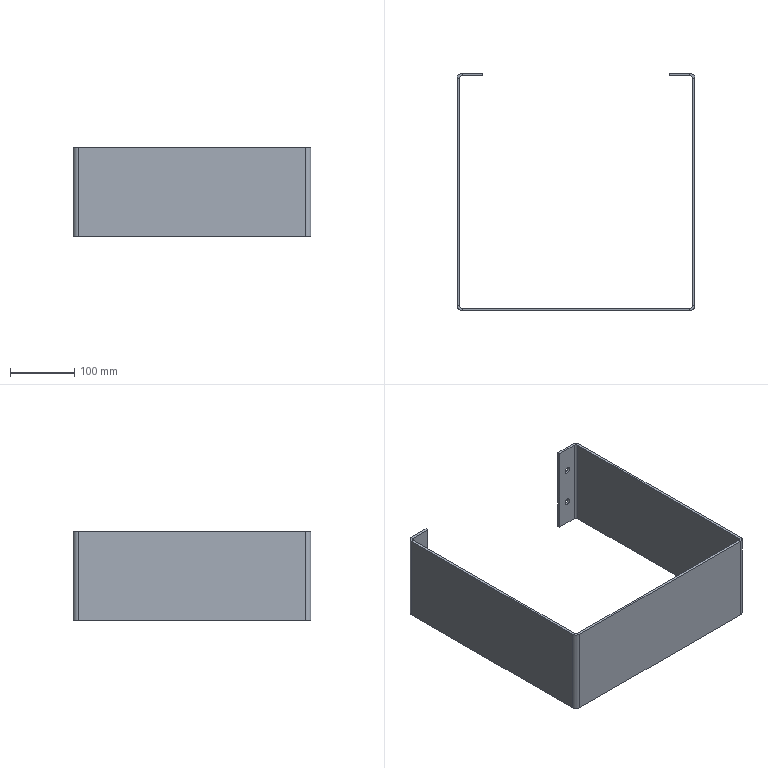Part | SolidWorks | features EdgeFlange 3, FlatPattern 1, ICE 1, SMBaseFlange 1, SheetMetal 1 | 1 solid | 46 faces | box 370 x 370 x 140 mm | volume 650415 mm3 | plane 30 | cylinder 16 | commonest cylinder face diameters 10 x8 8 x4 16 x4
STEP:
#1=CARTESIAN_POINT('',(-162.,366.,25.));
#2=VERTEX_POINT('',#1);
#3=CARTESIAN_POINT('',(-162.,366.,35.));
#4=VERTEX_POINT('',#3);
#5=CARTESIAN_POINT('',(-162.,366.,30.));
#6=DIRECTION('',(0.,1.,0.));
#7=DIRECTION('',(-1.,0.,0.));
#8=AXIS2_PLACEMENT_3D('',#5,#6,#7);
#9=CIRCLE('',#8,5.);
#10=EDGE_CURVE('',#2,#4,#9,.T.);
#11=ORIENTED_EDGE('',*,*,#10,.F.);
#12=CARTESIAN_POINT('',(-162.,370.,25.));
#13=VERTEX_POINT('',#12);
#14=CARTESIAN_POINT('',(-162.,280.,25.));
#15=DIRECTION('',(0.,1.,0.));
#16=VECTOR('',#15,1000.);
#17=LINE('',#14,#16);
#18=EDGE_CURVE('',#2,#13,#17,.T.);
#19=ORIENTED_EDGE('',*,*,#18,.T.);
#20=CARTESIAN_POINT('',(-162.,370.,35.));
#21=VERTEX_POINT('',#20);
#22=CARTESIAN_POINT('',(-162.,370.,30.));
#23=DIRECTION('',(0.,1.,0.));
#24=DIRECTION('',(0.,0.,-1.));
#25=AXIS2_PLACEMENT_3D('',#22,#23,#24);
#26=CIRCLE('',#25,5.);
#27=EDGE_CURVE('',#13,#21,#26,.T.);
#28=ORIENTED_EDGE('',*,*,#27,.T.);
#29=CARTESIAN_POINT('',(-162.,280.,35.));
#30=DIRECTION('',(0.,1.,0.));
#31=VECTOR('',#30,1000.);
#32=LINE('',#29,#31);
#33=EDGE_CURVE('',#4,#21,#32,.T.);
#34=ORIENTED_EDGE('',*,*,#33,.F.);
#35=EDGE_LOOP('',(#11,#19,#28,#34));
#36=FACE_OUTER_BOUND('',#35,.T.);
#37=CARTESIAN_POINT('',(-162.,280.,30.));
#38=DIRECTION('',(0.,1.,0.));
#39=DIRECTION('',(0.,0.,1.));
#40=AXIS2_PLACEMENT_3D('',#37,#38,#39);
#41=CYLINDRICAL_SURFACE('',#40,5.);
#42=ADVANCED_FACE('',(#36),#41,.F.);
#43=CARTESIAN_POINT('',(-162.,366.,-35.));
#44=VERTEX_POINT('',#43);
#45=CARTESIAN_POINT('',(-162.,366.,-25.));
#46=VERTEX_POINT('',#45);
#47=CARTESIAN_POINT('',(-162.,366.,-30.));
#48=DIRECTION('',(0.,1.,0.));
#49=DIRECTION('',(-1.,0.,0.));
#50=AXIS2_PLACEMENT_3D('',#47,#48,#49);
#51=CIRCLE('',#50,5.);
#52=EDGE_CURVE('',#44,#46,#51,.T.);
#53=ORIENTED_EDGE('',*,*,#52,.F.);
#54=CARTESIAN_POINT('',(-162.,370.,-35.));
#55=VERTEX_POINT('',#54);
#56=CARTESIAN_POINT('',(-162.,280.,-35.));
#57=DIRECTION('',(0.,1.,0.));
#58=VECTOR('',#57,1000.);
#59=LINE('',#56,#58);
#60=EDGE_CURVE('',#44,#55,#59,.T.);
#61=ORIENTED_EDGE('',*,*,#60,.T.);
#62=CARTESIAN_POINT('',(-162.,370.,-25.));
#63=VERTEX_POINT('',#62);
#64=CARTESIAN_POINT('',(-162.,370.,-30.));
#65=DIRECTION('',(0.,1.,0.));
#66=DIRECTION('',(0.,0.,1.));
#67=AXIS2_PLACEMENT_3D('',#64,#65,#66);
#68=CIRCLE('',#67,5.);
#69=EDGE_CURVE('',#55,#63,#68,.T.);
#70=ORIENTED_EDGE('',*,*,#69,.T.);
#71=CARTESIAN_POINT('',(-162.,280.,-25.));
#72=DIRECTION('',(0.,1.,0.));
#73=VECTOR('',#72,1000.);
#74=LINE('',#71,#73);
#75=EDGE_CURVE('',#46,#63,#74,.T.);
#76=ORIENTED_EDGE('',*,*,#75,.F.);
#77=EDGE_LOOP('',(#53,#61,#70,#76));
#78=FACE_OUTER_BOUND('',#77,.T.);
#79=CARTESIAN_POINT('',(-162.,280.,-30.));
#80=DIRECTION('',(0.,1.,0.));
#81=DIRECTION('',(0.,0.,1.));
#82=AXIS2_PLACEMENT_3D('',#79,#80,#81);
#83=CYLINDRICAL_SURFACE('',#82,5.);
#84=ADVANCED_FACE('',(#78),#83,.F.);
#85=CARTESIAN_POINT('',(162.,366.,-35.));
#86=VERTEX_POINT('',#85);
#87=CARTESIAN_POINT('',(162.,366.,-25.));
#88=VERTEX_POINT('',#87);
#89=CARTESIAN_POINT('',(162.,366.,-30.));
#90=DIRECTION('',(0.,1.,0.));
#91=DIRECTION('',(-1.,0.,0.));
#92=AXIS2_PLACEMENT_3D('',#89,#90,#91);
#93=CIRCLE('',#92,5.);
#94=EDGE_CURVE('',#86,#88,#93,.T.);
#95=ORIENTED_EDGE('',*,*,#94,.F.);
#96=CARTESIAN_POINT('',(162.,370.,-35.));
#97=VERTEX_POINT('',#96);
#98=CARTESIAN_POINT('',(162.,280.,-35.));
#99=DIRECTION('',(0.,1.,0.));
#100=VECTOR('',#99,1000.);
#101=LINE('',#98,#100);
#102=EDGE_CURVE('',#86,#97,#101,.T.);
#103=ORIENTED_EDGE('',*,*,#102,.T.);
#104=CARTESIAN_POINT('',(162.,370.,-25.));
#105=VERTEX_POINT('',#104);
#106=CARTESIAN_POINT('',(162.,370.,-30.));
#107=DIRECTION('',(0.,1.,0.));
#108=DIRECTION('',(0.,0.,-1.));
#109=AXIS2_PLACEMENT_3D('',#106,#107,#108);
#110=CIRCLE('',#109,5.);
#111=EDGE_CURVE('',#97,#105,#110,.T.);
#112=ORIENTED_EDGE('',*,*,#111,.T.);
#113=CARTESIAN_POINT('',(162.,280.,-25.));
#114=DIRECTION('',(0.,1.,0.));
#115=VECTOR('',#114,1000.);
#116=LINE('',#113,#115);
#117=EDGE_CURVE('',#88,#105,#116,.T.);
#118=ORIENTED_EDGE('',*,*,#117,.F.);
#119=EDGE_LOOP('',(#95,#103,#112,#118));
#120=FACE_OUTER_BOUND('',#119,.T.);
#121=CARTESIAN_POINT('',(162.,280.,-30.));
#122=DIRECTION('',(0.,1.,0.));
#123=DIRECTION('',(0.,0.,1.));
#124=AXIS2_PLACEMENT_3D('',#121,#122,#123);
#125=CYLINDRICAL_SURFACE('',#124,5.);
#126=ADVANCED_FACE('',(#120),#125,.F.);
#127=CARTESIAN_POINT('',(162.,366.,25.));
#128=VERTEX_POINT('',#127);
#129=CARTESIAN_POINT('',(162.,366.,35.));
#130=VERTEX_POINT('',#129);
#131=CARTESIAN_POINT('',(162.,366.,30.));
#132=DIRECTION('',(0.,1.,0.));
#133=DIRECTION('',(-1.,0.,0.));
#134=AXIS2_PLACEMENT_3D('',#131,#132,#133);
#135=CIRCLE('',#134,5.);
#136=EDGE_CURVE('',#128,#130,#135,.T.);
#137=ORIENTED_EDGE('',*,*,#136,.F.);
#138=CARTESIAN_POINT('',(162.,370.,25.));
#139=VERTEX_POINT('',#138);
#140=CARTESIAN_POINT('',(162.,280.,25.));
#141=DIRECTION('',(0.,1.,0.));
#142=VECTOR('',#141,1000.);
#143=LINE('',#140,#142);
#144=EDGE_CURVE('',#128,#139,#143,.T.);
#145=ORIENTED_EDGE('',*,*,#144,.T.);
#146=CARTESIAN_POINT('',(162.,370.,35.));
#147=VERTEX_POINT('',#146);
#148=CARTESIAN_POINT('',(162.,370.,30.));
#149=DIRECTION('',(0.,1.,0.));
#150=DIRECTION('',(0.,0.,1.));
#151=AXIS2_PLACEMENT_3D('',#148,#149,#150);
#152=CIRCLE('',#151,5.);
#153=EDGE_CURVE('',#139,#147,#152,.T.);
#154=ORIENTED_EDGE('',*,*,#153,.T.);
#155=CARTESIAN_POINT('',(162.,280.,35.));
#156=DIRECTION('',(0.,1.,0.));
#157=VECTOR('',#156,1000.);
#158=LINE('',#155,#157);
#159=EDGE_CURVE('',#130,#147,#158,.T.);
#160=ORIENTED_EDGE('',*,*,#159,.F.);
#161=EDGE_LOOP('',(#137,#145,#154,#160));
#162=FACE_OUTER_BOUND('',#161,.T.);
#163=CARTESIAN_POINT('',(162.,280.,30.));
#164=DIRECTION('',(0.,1.,0.));
#165=DIRECTION('',(0.,0.,1.));
#166=AXIS2_PLACEMENT_3D('',#163,#164,#165);
#167=CYLINDRICAL_SURFACE('',#166,5.);
#168=ADVANCED_FACE('',(#162),#167,.F.);
#169=CARTESIAN_POINT('',(181.,362.,70.));
#170=VERTEX_POINT('',#169);
#171=CARTESIAN_POINT('',(185.,362.,70.));
#172=VERTEX_POINT('',#171);
#173=CARTESIAN_POINT('',(181.,362.,70.));
#174=DIRECTION('',(1.,0.,0.));
#175=VECTOR('',#174,1000.);
#176=LINE('',#173,#175);
#177=EDGE_CURVE('',#170,#172,#176,.T.);
#178=ORIENTED_EDGE('',*,*,#177,.F.);
#179=CARTESIAN_POINT('',(181.,8.,70.));
#180=VERTEX_POINT('',#179);
#181=CARTESIAN_POINT('',(181.,4.,70.));
#182=DIRECTION('',(0.,-1.,0.));
#183=VECTOR('',#182,1000.);
#184=LINE('',#181,#183);
#185=EDGE_CURVE('',#170,#180,#184,.T.);
#186=ORIENTED_EDGE('',*,*,#185,.T.);
#187=CARTESIAN_POINT('',(185.,8.,70.));
#188=VERTEX_POINT('',#187);
#189=CARTESIAN_POINT('',(185.,8.,70.));
#190=DIRECTION('',(1.,0.,0.));
#191=VECTOR('',#190,1000.);
#192=LINE('',#189,#191);
#193=EDGE_CURVE('',#180,#188,#192,.T.);
#194=ORIENTED_EDGE('',*,*,#193,.T.);
#195=CARTESIAN_POINT('',(185.,0.,70.));
#196=DIRECTION('',(0.,-1.,0.));
#197=VECTOR('',#196,1000.);
#198=LINE('',#195,#197);
#199=EDGE_CURVE('',#172,#188,#198,.T.);
#200=ORIENTED_EDGE('',*,*,#199,.F.);
#201=EDGE_LOOP('',(#178,#186,#194,#200));
#202=FACE_OUTER_BOUND('',#201,.T.);
#203=CARTESIAN_POINT('',(185.,4.,70.));
#204=DIRECTION('',(0.,0.,-1.));
#205=DIRECTION('',(-1.,0.,0.));
#206=AXIS2_PLACEMENT_3D('',#203,#204,#205);
#207=PLANE('',#206);
#208=ADVANCED_FACE('',(#202),#207,.F.);
#209=CARTESIAN_POINT('',(181.,362.,-70.));
#210=VERTEX_POINT('',#209);
#211=CARTESIAN_POINT('',(185.,362.,-70.));
#212=VERTEX_POINT('',#211);
#213=CARTESIAN_POINT('',(181.,362.,-70.));
#214=DIRECTION('',(1.,0.,0.));
#215=VECTOR('',#214,1000.);
#216=LINE('',#213,#215);
#217=EDGE_CURVE('',#210,#212,#216,.T.);
#218=ORIENTED_EDGE('',*,*,#217,.T.);
#219=CARTESIAN_POINT('',(185.,8.,-70.));
#220=VERTEX_POINT('',#219);
#221=CARTESIAN_POINT('',(185.,0.,-70.));
#222=DIRECTION('',(0.,1.,0.));
#223=VECTOR('',#222,1000.);
#224=LINE('',#221,#223);
#225=EDGE_CURVE('',#220,#212,#224,.T.);
#226=ORIENTED_EDGE('',*,*,#225,.F.);
#227=CARTESIAN_POINT('',(181.,8.,-70.));
#228=VERTEX_POINT('',#227);
#229=CARTESIAN_POINT('',(181.,8.,-70.));
#230=DIRECTION('',(1.,0.,0.));
#231=VECTOR('',#230,1000.);
#232=LINE('',#229,#231);
#233=EDGE_CURVE('',#228,#220,#232,.T.);
#234=ORIENTED_EDGE('',*,*,#233,.F.);
#235=CARTESIAN_POINT('',(181.,370.,-70.));
#236=DIRECTION('',(0.,1.,0.));
#237=VECTOR('',#236,1000.);
#238=LINE('',#235,#237);
#239=EDGE_CURVE('',#228,#210,#238,.T.);
#240=ORIENTED_EDGE('',*,*,#239,.T.);
#241=EDGE_LOOP('',(#218,#226,#234,#240));
#242=FACE_OUTER_BOUND('',#241,.T.);
#243=CARTESIAN_POINT('',(185.,370.,-70.));
#244=DIRECTION('',(0.,0.,1.));
#245=DIRECTION('',(0.,-1.,0.));
#246=AXIS2_PLACEMENT_3D('',#243,#244,#245);
#247=PLANE('',#246);
#248=ADVANCED_FACE('',(#242),#247,.F.);
#249=CARTESIAN_POINT('',(185.,362.,-70.));
#250=DIRECTION('',(0.,0.,1.));
#251=VECTOR('',#250,1000.);
#252=LINE('',#249,#251);
#253=EDGE_CURVE('',#212,#172,#252,.T.);
#254=ORIENTED_EDGE('',*,*,#253,.T.);
#255=ORIENTED_EDGE('',*,*,#199,.T.);
#256=CARTESIAN_POINT('',(185.,8.,70.));
#257=DIRECTION('',(0.,0.,1.));
#258=VECTOR('',#257,1000.);
#259=LINE('',#256,#258);
#260=EDGE_CURVE('',#220,#188,#259,.T.);
#261=ORIENTED_EDGE('',*,*,#260,.F.);
#262=ORIENTED_EDGE('',*,*,#225,.T.);
#263=EDGE_LOOP('',(#254,#255,#261,#262));
#264=FACE_OUTER_BOUND('',#263,.T.);
#265=CARTESIAN_POINT('',(185.,0.,0.));
#266=DIRECTION('',(-1.,0.,0.));
#267=DIRECTION('',(0.,-1.,0.));
#268=AXIS2_PLACEMENT_3D('',#265,#266,#267);
#269=PLANE('',#268);
#270=ADVANCED_FACE('',(#264),#269,.F.);
#271=ORIENTED_EDGE('',*,*,#185,.F.);
#272=CARTESIAN_POINT('',(181.,362.,-70.));
#273=DIRECTION('',(0.,0.,1.));
#274=VECTOR('',#273,1000.);
#275=LINE('',#272,#274);
#276=EDGE_CURVE('',#210,#170,#275,.T.);
#277=ORIENTED_EDGE('',*,*,#276,.F.);
#278=ORIENTED_EDGE('',*,*,#239,.F.);
#279=CARTESIAN_POINT('',(181.,8.,70.));
#280=DIRECTION('',(0.,0.,-1.));
#281=VECTOR('',#280,1000.);
#282=LINE('',#279,#281);
#283=EDGE_CURVE('',#180,#228,#282,.T.);
#284=ORIENTED_EDGE('',*,*,#283,.F.);
#285=EDGE_LOOP('',(#271,#277,#278,#284));
#286=FACE_OUTER_BOUND('',#285,.T.);
#287=CARTESIAN_POINT('',(181.,0.,0.));
#288=DIRECTION('',(-1.,0.,0.));
#289=DIRECTION('',(0.,-1.,0.));
#290=AXIS2_PLACEMENT_3D('',#287,#288,#289);
#291=PLANE('',#290);
#292=ADVANCED_FACE('',(#286),#291,.T.);
#293=CARTESIAN_POINT('',(-181.,362.,70.));
#294=VERTEX_POINT('',#293);
#295=CARTESIAN_POINT('',(-185.,362.,70.));
#296=VERTEX_POINT('',#295);
#297=CARTESIAN_POINT('',(-181.,362.,70.));
#298=DIRECTION('',(-1.,0.,0.));
#299=VECTOR('',#298,1000.);
#300=LINE('',#297,#299);
#301=EDGE_CURVE('',#294,#296,#300,.T.);
#302=ORIENTED_EDGE('',*,*,#301,.T.);
#303=CARTESIAN_POINT('',(-185.,8.,70.));
#304=VERTEX_POINT('',#303);
#305=CARTESIAN_POINT('',(-185.,0.,70.));
#306=DIRECTION('',(0.,1.,0.));
#307=VECTOR('',#306,1000.);
#308=LINE('',#305,#307);
#309=EDGE_CURVE('',#304,#296,#308,.T.);
#310=ORIENTED_EDGE('',*,*,#309,.F.);
#311=CARTESIAN_POINT('',(-181.,8.,70.));
#312=VERTEX_POINT('',#311);
#313=CARTESIAN_POINT('',(-181.,8.,70.));
#314=DIRECTION('',(-1.,0.,0.));
#315=VECTOR('',#314,1000.);
#316=LINE('',#313,#315);
#317=EDGE_CURVE('',#312,#304,#316,.T.);
#318=ORIENTED_EDGE('',*,*,#317,.F.);
#319=CARTESIAN_POINT('',(-181.,4.,70.));
#320=DIRECTION('',(0.,1.,0.));
#321=VECTOR('',#320,1000.);
#322=LINE('',#319,#321);
#323=EDGE_CURVE('',#312,#294,#322,.T.);
#324=ORIENTED_EDGE('',*,*,#323,.T.);
#325=EDGE_LOOP('',(#302,#310,#318,#324));
#326=FACE_OUTER_BOUND('',#325,.T.);
#327=CARTESIAN_POINT('',(-185.,4.,70.));
#328=DIRECTION('',(0.,0.,-1.));
#329=DIRECTION('',(-1.,0.,0.));
#330=AXIS2_PLACEMENT_3D('',#327,#328,#329);
#331=PLANE('',#330);
#332=ADVANCED_FACE('',(#326),#331,.F.);
#333=CARTESIAN_POINT('',(-181.,362.,-70.));
#334=VERTEX_POINT('',#333);
#335=CARTESIAN_POINT('',(-185.,362.,-70.));
#336=VERTEX_POINT('',#335);
#337=CARTESIAN_POINT('',(-181.,362.,-70.));
#338=DIRECTION('',(-1.,0.,0.));
#339=VECTOR('',#338,1000.);
#340=LINE('',#337,#339);
#341=EDGE_CURVE('',#334,#336,#340,.T.);
#342=ORIENTED_EDGE('',*,*,#341,.F.);
#343=CARTESIAN_POINT('',(-181.,8.,-70.));
#344=VERTEX_POINT('',#343);
#345=CARTESIAN_POINT('',(-181.,370.,-70.));
#346=DIRECTION('',(0.,-1.,0.));
#347=VECTOR('',#346,1000.);
#348=LINE('',#345,#347);
#349=EDGE_CURVE('',#334,#344,#348,.T.);
#350=ORIENTED_EDGE('',*,*,#349,.T.);
#351=CARTESIAN_POINT('',(-185.,8.,-70.));
#352=VERTEX_POINT('',#351);
#353=CARTESIAN_POINT('',(-185.,8.,-70.));
#354=DIRECTION('',(-1.,0.,0.));
#355=VECTOR('',#354,1000.);
#356=LINE('',#353,#355);
#357=EDGE_CURVE('',#344,#352,#356,.T.);
#358=ORIENTED_EDGE('',*,*,#357,.T.);
#359=CARTESIAN_POINT('',(-185.,0.,-70.));
#360=DIRECTION('',(0.,-1.,0.));
#361=VECTOR('',#360,1000.);
#362=LINE('',#359,#361);
#363=EDGE_CURVE('',#336,#352,#362,.T.);
#364=ORIENTED_EDGE('',*,*,#363,.F.);
#365=EDGE_LOOP('',(#342,#350,#358,#364));
#366=FACE_OUTER_BOUND('',#365,.T.);
#367=CARTESIAN_POINT('',(-185.,370.,-70.));
#368=DIRECTION('',(0.,0.,1.));
#369=DIRECTION('',(0.,-1.,0.));
#370=AXIS2_PLACEMENT_3D('',#367,#368,#369);
#371=PLANE('',#370);
#372=ADVANCED_FACE('',(#366),#371,.F.);
#373=ORIENTED_EDGE('',*,*,#309,.T.);
#374=CARTESIAN_POINT('',(-185.,362.,70.));
#375=DIRECTION('',(0.,0.,-1.));
#376=VECTOR('',#375,1000.);
#377=LINE('',#374,#376);
#378=EDGE_CURVE('',#296,#336,#377,.T.);
#379=ORIENTED_EDGE('',*,*,#378,.T.);
#380=ORIENTED_EDGE('',*,*,#363,.T.);
#381=CARTESIAN_POINT('',(-185.,8.,0.));
#382=DIRECTION('',(0.,0.,1.));
#383=VECTOR('',#382,1000.);
#384=LINE('',#381,#383);
#385=EDGE_CURVE('',#352,#304,#384,.T.);
#386=ORIENTED_EDGE('',*,*,#385,.T.);
#387=EDGE_LOOP('',(#373,#379,#380,#386));
#388=FACE_OUTER_BOUND('',#387,.T.);
#389=CARTESIAN_POINT('',(-185.,0.,0.));
#390=DIRECTION('',(-1.,0.,0.));
#391=DIRECTION('',(0.,-1.,0.));
#392=AXIS2_PLACEMENT_3D('',#389,#390,#391);
#393=PLANE('',#392);
#394=ADVANCED_FACE('',(#388),#393,.T.);
#395=CARTESIAN_POINT('',(-181.,362.,70.));
#396=DIRECTION('',(0.,0.,-1.));
#397=VECTOR('',#396,1000.);
#398=LINE('',#395,#397);
#399=EDGE_CURVE('',#294,#334,#398,.T.);
#400=ORIENTED_EDGE('',*,*,#399,.F.);
#401=ORIENTED_EDGE('',*,*,#323,.F.);
#402=CARTESIAN_POINT('',(-181.,8.,-70.));
#403=DIRECTION('',(0.,0.,1.));
#404=VECTOR('',#403,1000.);
#405=LINE('',#402,#404);
#406=EDGE_CURVE('',#344,#312,#405,.T.);
#407=ORIENTED_EDGE('',*,*,#406,.F.);
#408=ORIENTED_EDGE('',*,*,#349,.F.);
#409=EDGE_LOOP('',(#400,#401,#407,#408));
#410=FACE_OUTER_BOUND('',#409,.T.);
#411=CARTESIAN_POINT('',(-181.,0.,0.));
#412=DIRECTION('',(-1.,0.,0.));
#413=DIRECTION('',(0.,-1.,0.));
#414=AXIS2_PLACEMENT_3D('',#411,#412,#413);
#415=PLANE('',#414);
#416=ADVANCED_FACE('',(#410),#415,.F.);
#417=CARTESIAN_POINT('',(177.,4.,-70.));
#418=VERTEX_POINT('',#417);
#419=CARTESIAN_POINT('',(177.,0.,-70.));
#420=VERTEX_POINT('',#419);
#421=CARTESIAN_POINT('',(177.,4.,-70.));
#422=DIRECTION('',(0.,-1.,0.));
#423=VECTOR('',#422,1000.);
#424=LINE('',#421,#423);
#425=EDGE_CURVE('',#418,#420,#424,.T.);
#426=ORIENTED_EDGE('',*,*,#425,.T.);
#427=CARTESIAN_POINT('',(-177.,0.,-70.));
#428=VERTEX_POINT('',#427);
#429=CARTESIAN_POINT('',(-185.,0.,-70.));
#430=DIRECTION('',(-1.,0.,0.));
#431=VECTOR('',#430,1000.);
#432=LINE('',#429,#431);
#433=EDGE_CURVE('',#420,#428,#432,.T.);
#434=ORIENTED_EDGE('',*,*,#433,.T.);
#435=CARTESIAN_POINT('',(-177.,4.,-70.));
#436=VERTEX_POINT('',#435);
#437=CARTESIAN_POINT('',(-177.,4.,-70.));
#438=DIRECTION('',(0.,-1.,0.));
#439=VECTOR('',#438,1000.);
#440=LINE('',#437,#439);
#441=EDGE_CURVE('',#436,#428,#440,.T.);
#442=ORIENTED_EDGE('',*,*,#441,.F.);
#443=CARTESIAN_POINT('',(-185.,4.,-70.));
#444=DIRECTION('',(-1.,0.,0.));
#445=VECTOR('',#444,1000.);
#446=LINE('',#443,#445);
#447=EDGE_CURVE('',#418,#436,#446,.T.);
#448=ORIENTED_EDGE('',*,*,#447,.F.);
#449=EDGE_LOOP('',(#426,#434,#442,#448));
#450=FACE_OUTER_BOUND('',#449,.T.);
#451=CARTESIAN_POINT('',(-185.,4.,-70.));
#452=DIRECTION('',(0.,0.,1.));
#453=DIRECTION('',(1.,0.,0.));
#454=AXIS2_PLACEMENT_3D('',#451,#452,#453);
#455=PLANE('',#454);
#456=ADVANCED_FACE('',(#450),#455,.F.);
#457=CARTESIAN_POINT('',(177.,4.,70.));
#458=VERTEX_POINT('',#457);
#459=CARTESIAN_POINT('',(177.,0.,70.));
#460=VERTEX_POINT('',#459);
#461=CARTESIAN_POINT('',(177.,4.,70.));
#462=DIRECTION('',(0.,-1.,0.));
#463=VECTOR('',#462,1000.);
#464=LINE('',#461,#463);
#465=EDGE_CURVE('',#458,#460,#464,.T.);
#466=ORIENTED_EDGE('',*,*,#465,.F.);
#467=CARTESIAN_POINT('',(-177.,4.,70.));
#468=VERTEX_POINT('',#467);
#469=CARTESIAN_POINT('',(-185.,4.,70.));
#470=DIRECTION('',(1.,0.,0.));
#471=VECTOR('',#470,1000.);
#472=LINE('',#469,#471);
#473=EDGE_CURVE('',#468,#458,#472,.T.);
#474=ORIENTED_EDGE('',*,*,#473,.F.);
#475=CARTESIAN_POINT('',(-177.,0.,70.));
#476=VERTEX_POINT('',#475);
#477=CARTESIAN_POINT('',(-177.,4.,70.));
#478=DIRECTION('',(0.,-1.,0.));
#479=VECTOR('',#478,1000.);
#480=LINE('',#477,#479);
#481=EDGE_CURVE('',#468,#476,#480,.T.);
#482=ORIENTED_EDGE('',*,*,#481,.T.);
#483=CARTESIAN_POINT('',(-185.,0.,70.));
#484=DIRECTION('',(1.,0.,0.));
#485=VECTOR('',#484,1000.);
#486=LINE('',#483,#485);
#487=EDGE_CURVE('',#476,#460,#486,.T.);
#488=ORIENTED_EDGE('',*,*,#487,.T.);
#489=EDGE_LOOP('',(#466,#474,#482,#488));
#490=FACE_OUTER_BOUND('',#489,.T.);
#491=CARTESIAN_POINT('',(-185.,4.,70.));
#492=DIRECTION('',(0.,0.,-1.));
#493=DIRECTION('',(-1.,0.,0.));
#494=AXIS2_PLACEMENT_3D('',#491,#492,#493);
#495=PLANE('',#494);
#496=ADVANCED_FACE('',(#490),#495,.F.);
#497=ORIENTED_EDGE('',*,*,#473,.T.);
#498=CARTESIAN_POINT('',(177.,4.,-70.));
#499=DIRECTION('',(0.,0.,1.));
#500=VECTOR('',#499,1000.);
#501=LINE('',#498,#500);
#502=EDGE_CURVE('',#418,#458,#501,.T.);
#503=ORIENTED_EDGE('',*,*,#502,.F.);
#504=ORIENTED_EDGE('',*,*,#447,.T.);
#505=CARTESIAN_POINT('',(-177.,4.,70.));
#506=DIRECTION('',(0.,0.,-1.));
#507=VECTOR('',#506,1000.);
#508=LINE('',#505,#507);
#509=EDGE_CURVE('',#468,#436,#508,.T.);
#510=ORIENTED_EDGE('',*,*,#509,.F.);
#511=EDGE_LOOP('',(#497,#503,#504,#510));
#512=FACE_OUTER_BOUND('',#511,.T.);
#513=CARTESIAN_POINT('',(0.,4.,0.));
#514=DIRECTION('',(0.,1.,0.));
#515=DIRECTION('',(0.,0.,1.));
#516=AXIS2_PLACEMENT_3D('',#513,#514,#515);
#517=PLANE('',#516);
#518=ADVANCED_FACE('',(#512),#517,.T.);
#519=CARTESIAN_POINT('',(177.,0.,-70.));
#520=DIRECTION('',(0.,0.,1.));
#521=VECTOR('',#520,1000.);
#522=LINE('',#519,#521);
#523=EDGE_CURVE('',#420,#460,#522,.T.);
#524=ORIENTED_EDGE('',*,*,#523,.T.);
#525=ORIENTED_EDGE('',*,*,#487,.F.);
#526=CARTESIAN_POINT('',(-177.,0.,70.));
#527=DIRECTION('',(0.,0.,-1.));
#528=VECTOR('',#527,1000.);
#529=LINE('',#526,#528);
#530=EDGE_CURVE('',#476,#428,#529,.T.);
#531=ORIENTED_EDGE('',*,*,#530,.T.);
#532=ORIENTED_EDGE('',*,*,#433,.F.);
#533=EDGE_LOOP('',(#524,#525,#531,#532));
#534=FACE_OUTER_BOUND('',#533,.T.);
#535=CARTESIAN_POINT('',(0.,0.,0.));
#536=DIRECTION('',(0.,1.,0.));
#537=DIRECTION('',(0.,0.,1.));
#538=AXIS2_PLACEMENT_3D('',#535,#536,#537);
#539=PLANE('',#538);
#540=ADVANCED_FACE('',(#534),#539,.F.);
#541=ORIENTED_EDGE('',*,*,#357,.F.);
#542=CARTESIAN_POINT('',(-177.,8.,-70.));
#543=DIRECTION('',(0.,0.,-1.));
#544=DIRECTION('',(1.,0.,0.));
#545=AXIS2_PLACEMENT_3D('',#542,#543,#544);
#546=CIRCLE('',#545,4.);
#547=EDGE_CURVE('',#436,#344,#546,.T.);
#548=ORIENTED_EDGE('',*,*,#547,.F.);
#549=ORIENTED_EDGE('',*,*,#441,.T.);
#550=CARTESIAN_POINT('',(-177.,8.,-70.));
#551=DIRECTION('',(0.,0.,-1.));
#552=DIRECTION('',(1.,0.,0.));
#553=AXIS2_PLACEMENT_3D('',#550,#551,#552);
#554=CIRCLE('',#553,8.);
#555=EDGE_CURVE('',#428,#352,#554,.T.);
#556=ORIENTED_EDGE('',*,*,#555,.T.);
#557=EDGE_LOOP('',(#541,#548,#549,#556));
#558=FACE_OUTER_BOUND('',#557,.T.);
#559=CARTESIAN_POINT('',(-177.,8.,-70.));
#560=DIRECTION('',(0.,0.,-1.));
#561=DIRECTION('',(-1.,0.,0.));
#562=AXIS2_PLACEMENT_3D('',#559,#560,#561);
#563=PLANE('',#562);
#564=ADVANCED_FACE('',(#558),#563,.T.);
#565=CARTESIAN_POINT('',(-177.,8.,70.));
#566=DIRECTION('',(0.,0.,1.));
#567=DIRECTION('',(1.,0.,0.));
#568=AXIS2_PLACEMENT_3D('',#565,#566,#567);
#569=CIRCLE('',#568,4.);
#570=EDGE_CURVE('',#312,#468,#569,.T.);
#571=ORIENTED_EDGE('',*,*,#570,.F.);
#572=ORIENTED_EDGE('',*,*,#317,.T.);
#573=CARTESIAN_POINT('',(-177.,8.,70.));
#574=DIRECTION('',(0.,0.,1.));
#575=DIRECTION('',(1.,0.,0.));
#576=AXIS2_PLACEMENT_3D('',#573,#574,#575);
#577=CIRCLE('',#576,8.);
#578=EDGE_CURVE('',#304,#476,#577,.T.);
#579=ORIENTED_EDGE('',*,*,#578,.T.);
#580=ORIENTED_EDGE('',*,*,#481,.F.);
#581=EDGE_LOOP('',(#571,#572,#579,#580));
#582=FACE_OUTER_BOUND('',#581,.T.);
#583=CARTESIAN_POINT('',(-177.,8.,70.));
#584=DIRECTION('',(0.,0.,-1.));
#585=DIRECTION('',(-1.,0.,0.));
#586=AXIS2_PLACEMENT_3D('',#583,#584,#585);
#587=PLANE('',#586);
#588=ADVANCED_FACE('',(#582),#587,.F.);
#589=ORIENTED_EDGE('',*,*,#530,.F.);
#590=ORIENTED_EDGE('',*,*,#578,.F.);
#591=ORIENTED_EDGE('',*,*,#385,.F.);
#592=ORIENTED_EDGE('',*,*,#555,.F.);
#593=EDGE_LOOP('',(#589,#590,#591,#592));
#594=FACE_OUTER_BOUND('',#593,.T.);
#595=CARTESIAN_POINT('',(-177.,8.,70.));
#596=DIRECTION('',(0.,0.,1.));
#597=DIRECTION('',(-1.,0.,0.));
#598=AXIS2_PLACEMENT_3D('',#595,#596,#597);
#599=CYLINDRICAL_SURFACE('',#598,8.);
#600=ADVANCED_FACE('',(#594),#599,.T.);
#601=ORIENTED_EDGE('',*,*,#509,.T.);
#602=ORIENTED_EDGE('',*,*,#547,.T.);
#603=ORIENTED_EDGE('',*,*,#406,.T.);
#604=ORIENTED_EDGE('',*,*,#570,.T.);
#605=EDGE_LOOP('',(#601,#602,#603,#604));
#606=FACE_OUTER_BOUND('',#605,.T.);
#607=CARTESIAN_POINT('',(-177.,8.,70.));
#608=DIRECTION('',(0.,0.,1.));
#609=DIRECTION('',(-1.,0.,0.));
#610=AXIS2_PLACEMENT_3D('',#607,#608,#609);
#611=CYLINDRICAL_SURFACE('',#610,4.);
#612=ADVANCED_FACE('',(#606),#611,.F.);
#613=ORIENTED_EDGE('',*,*,#193,.F.);
#614=CARTESIAN_POINT('',(177.,8.,70.));
#615=DIRECTION('',(0.,0.,1.));
#616=DIRECTION('',(-1.,0.,0.));
#617=AXIS2_PLACEMENT_3D('',#614,#615,#616);
#618=CIRCLE('',#617,4.);
#619=EDGE_CURVE('',#458,#180,#618,.T.);
#620=ORIENTED_EDGE('',*,*,#619,.F.);
#621=ORIENTED_EDGE('',*,*,#465,.T.);
#622=CARTESIAN_POINT('',(177.,8.,70.));
#623=DIRECTION('',(0.,0.,1.));
#624=DIRECTION('',(-1.,0.,0.));
#625=AXIS2_PLACEMENT_3D('',#622,#623,#624);
#626=CIRCLE('',#625,8.);
#627=EDGE_CURVE('',#460,#188,#626,.T.);
#628=ORIENTED_EDGE('',*,*,#627,.T.);
#629=EDGE_LOOP('',(#613,#620,#621,#628));
#630=FACE_OUTER_BOUND('',#629,.T.);
#631=CARTESIAN_POINT('',(177.,8.,70.));
#632=DIRECTION('',(0.,0.,1.));
#633=DIRECTION('',(1.,0.,0.));
#634=AXIS2_PLACEMENT_3D('',#631,#632,#633);
#635=PLANE('',#634);
#636=ADVANCED_FACE('',(#630),#635,.T.);
#637=CARTESIAN_POINT('',(177.,8.,-70.));
#638=DIRECTION('',(0.,0.,-1.));
#639=DIRECTION('',(-1.,0.,0.));
#640=AXIS2_PLACEMENT_3D('',#637,#638,#639);
#641=CIRCLE('',#640,4.);
#642=EDGE_CURVE('',#228,#418,#641,.T.);
#643=ORIENTED_EDGE('',*,*,#642,.F.);
#644=ORIENTED_EDGE('',*,*,#233,.T.);
#645=CARTESIAN_POINT('',(177.,8.,-70.));
#646=DIRECTION('',(0.,0.,-1.));
#647=DIRECTION('',(-1.,0.,0.));
#648=AXIS2_PLACEMENT_3D('',#645,#646,#647);
#649=CIRCLE('',#648,8.);
#650=EDGE_CURVE('',#220,#420,#649,.T.);
#651=ORIENTED_EDGE('',*,*,#650,.T.);
#652=ORIENTED_EDGE('',*,*,#425,.F.);
#653=EDGE_LOOP('',(#643,#644,#651,#652));
#654=FACE_OUTER_BOUND('',#653,.T.);
#655=CARTESIAN_POINT('',(177.,8.,-70.));
#656=DIRECTION('',(0.,0.,1.));
#657=DIRECTION('',(1.,0.,0.));
#658=AXIS2_PLACEMENT_3D('',#655,#656,#657);
#659=PLANE('',#658);
#660=ADVANCED_FACE('',(#654),#659,.F.);
#661=ORIENTED_EDGE('',*,*,#523,.F.);
#662=ORIENTED_EDGE('',*,*,#650,.F.);
#663=ORIENTED_EDGE('',*,*,#260,.T.);
#664=ORIENTED_EDGE('',*,*,#627,.F.);
#665=EDGE_LOOP('',(#661,#662,#663,#664));
#666=FACE_OUTER_BOUND('',#665,.T.);
#667=CARTESIAN_POINT('',(177.,8.,-70.));
#668=DIRECTION('',(0.,0.,-1.));
#669=DIRECTION('',(1.,0.,0.));
#670=AXIS2_PLACEMENT_3D('',#667,#668,#669);
#671=CYLINDRICAL_SURFACE('',#670,8.);
#672=ADVANCED_FACE('',(#666),#671,.T.);
#673=ORIENTED_EDGE('',*,*,#502,.T.);
#674=ORIENTED_EDGE('',*,*,#619,.T.);
#675=ORIENTED_EDGE('',*,*,#283,.T.);
#676=ORIENTED_EDGE('',*,*,#642,.T.);
#677=EDGE_LOOP('',(#673,#674,#675,#676));
#678=FACE_OUTER_BOUND('',#677,.T.);
#679=CARTESIAN_POINT('',(177.,8.,-70.));
#680=DIRECTION('',(0.,0.,-1.));
#681=DIRECTION('',(1.,0.,0.));
#682=AXIS2_PLACEMENT_3D('',#679,#680,#681);
#683=CYLINDRICAL_SURFACE('',#682,4.);
#684=ADVANCED_FACE('',(#678),#683,.F.);
#685=CARTESIAN_POINT('',(-177.,366.,-70.));
#686=VERTEX_POINT('',#685);
#687=CARTESIAN_POINT('',(-177.,370.,-70.));
#688=VERTEX_POINT('',#687);
#689=CARTESIAN_POINT('',(-177.,370.,-70.));
#690=DIRECTION('',(0.,1.,0.));
#691=VECTOR('',#690,1000.);
#692=LINE('',#689,#691);
#693=EDGE_CURVE('',#686,#688,#692,.T.);
#694=ORIENTED_EDGE('',*,*,#693,.F.);
#695=CARTESIAN_POINT('',(-177.,362.,-70.));
#696=DIRECTION('',(0.,0.,-1.));
#697=DIRECTION('',(1.,0.,0.));
#698=AXIS2_PLACEMENT_3D('',#695,#696,#697);
#699=CIRCLE('',#698,4.);
#700=EDGE_CURVE('',#334,#686,#699,.T.);
#701=ORIENTED_EDGE('',*,*,#700,.F.);
#702=ORIENTED_EDGE('',*,*,#341,.T.);
#703=CARTESIAN_POINT('',(-177.,362.,-70.));
#704=DIRECTION('',(0.,0.,-1.));
#705=DIRECTION('',(1.,0.,0.));
#706=AXIS2_PLACEMENT_3D('',#703,#704,#705);
#707=CIRCLE('',#706,8.);
#708=EDGE_CURVE('',#336,#688,#707,.T.);
#709=ORIENTED_EDGE('',*,*,#708,.T.);
#710=EDGE_LOOP('',(#694,#701,#702,#709));
#711=FACE_OUTER_BOUND('',#710,.T.);
#712=CARTESIAN_POINT('',(-177.,362.,-70.));
#713=DIRECTION('',(0.,0.,-1.));
#714=DIRECTION('',(-1.,0.,0.));
#715=AXIS2_PLACEMENT_3D('',#712,#713,#714);
#716=PLANE('',#715);
#717=ADVANCED_FACE('',(#711),#716,.T.);
#718=CARTESIAN_POINT('',(-177.,366.,70.));
#719=VERTEX_POINT('',#718);
#720=CARTESIAN_POINT('',(-177.,362.,70.));
#721=DIRECTION('',(0.,0.,1.));
#722=DIRECTION('',(1.,0.,0.));
#723=AXIS2_PLACEMENT_3D('',#720,#721,#722);
#724=CIRCLE('',#723,4.);
#725=EDGE_CURVE('',#719,#294,#724,.T.);
#726=ORIENTED_EDGE('',*,*,#725,.F.);
#727=CARTESIAN_POINT('',(-177.,370.,70.));
#728=VERTEX_POINT('',#727);
#729=CARTESIAN_POINT('',(-177.,366.,70.));
#730=DIRECTION('',(0.,1.,0.));
#731=VECTOR('',#730,1000.);
#732=LINE('',#729,#731);
#733=EDGE_CURVE('',#719,#728,#732,.T.);
#734=ORIENTED_EDGE('',*,*,#733,.T.);
#735=CARTESIAN_POINT('',(-177.,362.,70.));
#736=DIRECTION('',(0.,0.,1.));
#737=DIRECTION('',(1.,0.,0.));
#738=AXIS2_PLACEMENT_3D('',#735,#736,#737);
#739=CIRCLE('',#738,8.);
#740=EDGE_CURVE('',#728,#296,#739,.T.);
#741=ORIENTED_EDGE('',*,*,#740,.T.);
#742=ORIENTED_EDGE('',*,*,#301,.F.);
#743=EDGE_LOOP('',(#726,#734,#741,#742));
#744=FACE_OUTER_BOUND('',#743,.T.);
#745=CARTESIAN_POINT('',(-177.,362.,70.));
#746=DIRECTION('',(0.,0.,-1.));
#747=DIRECTION('',(-1.,0.,0.));
#748=AXIS2_PLACEMENT_3D('',#745,#746,#747);
#749=PLANE('',#748);
#750=ADVANCED_FACE('',(#744),#749,.F.);
#751=ORIENTED_EDGE('',*,*,#378,.F.);
#752=ORIENTED_EDGE('',*,*,#740,.F.);
#753=CARTESIAN_POINT('',(-177.,370.,0.));
#754=DIRECTION('',(0.,0.,1.));
#755=VECTOR('',#754,1000.);
#756=LINE('',#753,#755);
#757=EDGE_CURVE('',#688,#728,#756,.T.);
#758=ORIENTED_EDGE('',*,*,#757,.F.);
#759=ORIENTED_EDGE('',*,*,#708,.F.);
#760=EDGE_LOOP('',(#751,#752,#758,#759));
#761=FACE_OUTER_BOUND('',#760,.T.);
#762=CARTESIAN_POINT('',(-177.,362.,70.));
#763=DIRECTION('',(0.,0.,1.));
#764=DIRECTION('',(0.,1.,0.));
#765=AXIS2_PLACEMENT_3D('',#762,#763,#764);
#766=CYLINDRICAL_SURFACE('',#765,8.);
#767=ADVANCED_FACE('',(#761),#766,.T.);
#768=ORIENTED_EDGE('',*,*,#399,.T.);
#769=ORIENTED_EDGE('',*,*,#700,.T.);
#770=CARTESIAN_POINT('',(-177.,366.,-70.));
#771=DIRECTION('',(0.,0.,1.));
#772=VECTOR('',#771,1000.);
#773=LINE('',#770,#772);
#774=EDGE_CURVE('',#686,#719,#773,.T.);
#775=ORIENTED_EDGE('',*,*,#774,.T.);
#776=ORIENTED_EDGE('',*,*,#725,.T.);
#777=EDGE_LOOP('',(#768,#769,#775,#776));
#778=FACE_OUTER_BOUND('',#777,.T.);
#779=CARTESIAN_POINT('',(-177.,362.,70.));
#780=DIRECTION('',(0.,0.,1.));
#781=DIRECTION('',(0.,1.,0.));
#782=AXIS2_PLACEMENT_3D('',#779,#780,#781);
#783=CYLINDRICAL_SURFACE('',#782,4.);
#784=ADVANCED_FACE('',(#778),#783,.F.);
#785=CARTESIAN_POINT('',(-145.,370.,70.));
#786=VERTEX_POINT('',#785);
#787=CARTESIAN_POINT('',(-181.,370.,70.));
#788=DIRECTION('',(-1.,0.,0.));
#789=VECTOR('',#788,1000.);
#790=LINE('',#787,#789);
#791=EDGE_CURVE('',#786,#728,#790,.T.);
#792=ORIENTED_EDGE('',*,*,#791,.T.);
#793=ORIENTED_EDGE('',*,*,#733,.F.);
#794=CARTESIAN_POINT('',(-145.,366.,70.));
#795=VERTEX_POINT('',#794);
#796=CARTESIAN_POINT('',(0.,366.,70.));
#797=DIRECTION('',(-1.,0.,0.));
#798=VECTOR('',#797,1000.);
#799=LINE('',#796,#798);
#800=EDGE_CURVE('',#795,#719,#799,.T.);
#801=ORIENTED_EDGE('',*,*,#800,.F.);
#802=CARTESIAN_POINT('',(-145.,370.,70.));
#803=DIRECTION('',(0.,-1.,0.));
#804=VECTOR('',#803,1000.);
#805=LINE('',#802,#804);
#806=EDGE_CURVE('',#786,#795,#805,.T.);
#807=ORIENTED_EDGE('',*,*,#806,.F.);
#808=EDGE_LOOP('',(#792,#793,#801,#807));
#809=FACE_OUTER_BOUND('',#808,.T.);
#810=CARTESIAN_POINT('',(-181.,370.,70.));
#811=DIRECTION('',(0.,0.,1.));
#812=DIRECTION('',(1.,0.,0.));
#813=AXIS2_PLACEMENT_3D('',#810,#811,#812);
#814=PLANE('',#813);
#815=ADVANCED_FACE('',(#809),#814,.T.);
#816=CARTESIAN_POINT('',(-145.,366.,-70.));
#817=VERTEX_POINT('',#816);
#818=CARTESIAN_POINT('',(0.,366.,-70.));
#819=DIRECTION('',(1.,0.,0.));
#820=VECTOR('',#819,1000.);
#821=LINE('',#818,#820);
#822=EDGE_CURVE('',#686,#817,#821,.T.);
#823=ORIENTED_EDGE('',*,*,#822,.F.);
#824=ORIENTED_EDGE('',*,*,#693,.T.);
#825=CARTESIAN_POINT('',(-145.,370.,-70.));
#826=VERTEX_POINT('',#825);
#827=CARTESIAN_POINT('',(-145.,370.,-70.));
#828=DIRECTION('',(1.,0.,0.));
#829=VECTOR('',#828,1000.);
#830=LINE('',#827,#829);
#831=EDGE_CURVE('',#688,#826,#830,.T.);
#832=ORIENTED_EDGE('',*,*,#831,.T.);
#833=CARTESIAN_POINT('',(-145.,370.,-70.));
#834=DIRECTION('',(0.,-1.,0.));
#835=VECTOR('',#834,1000.);
#836=LINE('',#833,#835);
#837=EDGE_CURVE('',#826,#817,#836,.T.);
#838=ORIENTED_EDGE('',*,*,#837,.T.);
#839=EDGE_LOOP('',(#823,#824,#832,#838));
#840=FACE_OUTER_BOUND('',#839,.T.);
#841=CARTESIAN_POINT('',(-145.,370.,-70.));
#842=DIRECTION('',(0.,0.,-1.));
#843=DIRECTION('',(-1.,0.,0.));
#844=AXIS2_PLACEMENT_3D('',#841,#842,#843);
#845=PLANE('',#844);
#846=ADVANCED_FACE('',(#840),#845,.T.);
#847=CARTESIAN_POINT('',(-162.,370.,30.));
#848=DIRECTION('',(0.,1.,0.));
#849=DIRECTION('',(0.,0.,-1.));
#850=AXIS2_PLACEMENT_3D('',#847,#848,#849);
#851=CIRCLE('',#850,5.);
#852=EDGE_CURVE('',#21,#13,#851,.T.);
#853=ORIENTED_EDGE('',*,*,#852,.F.);
#854=ORIENTED_EDGE('',*,*,#27,.F.);
#855=EDGE_LOOP('',(#853,#854));
#856=FACE_BOUND('',#855,.T.);
#857=CARTESIAN_POINT('',(-162.,370.,-30.));
#858=DIRECTION('',(0.,1.,0.));
#859=DIRECTION('',(0.,0.,1.));
#860=AXIS2_PLACEMENT_3D('',#857,#858,#859);
#861=CIRCLE('',#860,5.);
#862=EDGE_CURVE('',#63,#55,#861,.T.);
#863=ORIENTED_EDGE('',*,*,#862,.F.);
#864=ORIENTED_EDGE('',*,*,#69,.F.);
#865=EDGE_LOOP('',(#863,#864));
#866=FACE_BOUND('',#865,.T.);
#867=ORIENTED_EDGE('',*,*,#831,.F.);
#868=ORIENTED_EDGE('',*,*,#757,.T.);
#869=ORIENTED_EDGE('',*,*,#791,.F.);
#870=CARTESIAN_POINT('',(-145.,370.,70.));
#871=DIRECTION('',(0.,0.,1.));
#872=VECTOR('',#871,1000.);
#873=LINE('',#870,#872);
#874=EDGE_CURVE('',#826,#786,#873,.T.);
#875=ORIENTED_EDGE('',*,*,#874,.F.);
#876=EDGE_LOOP('',(#867,#868,#869,#875));
#877=FACE_OUTER_BOUND('',#876,.T.);
#878=CARTESIAN_POINT('',(0.,370.,0.));
#879=DIRECTION('',(0.,1.,0.));
#880=DIRECTION('',(-1.,0.,0.));
#881=AXIS2_PLACEMENT_3D('',#878,#879,#880);
#882=PLANE('',#881);
#883=ADVANCED_FACE('',(#856,#866,#877),#882,.T.);
#884=CARTESIAN_POINT('',(-162.,366.,30.));
#885=DIRECTION('',(0.,1.,0.));
#886=DIRECTION('',(-1.,0.,0.));
#887=AXIS2_PLACEMENT_3D('',#884,#885,#886);
#888=CIRCLE('',#887,5.);
#889=EDGE_CURVE('',#4,#2,#888,.T.);
#890=ORIENTED_EDGE('',*,*,#889,.T.);
#891=ORIENTED_EDGE('',*,*,#10,.T.);
#892=EDGE_LOOP('',(#890,#891));
#893=FACE_BOUND('',#892,.T.);
#894=CARTESIAN_POINT('',(-162.,366.,-30.));
#895=DIRECTION('',(0.,1.,0.));
#896=DIRECTION('',(-1.,0.,0.));
#897=AXIS2_PLACEMENT_3D('',#894,#895,#896);
#898=CIRCLE('',#897,5.);
#899=EDGE_CURVE('',#46,#44,#898,.T.);
#900=ORIENTED_EDGE('',*,*,#899,.T.);
#901=ORIENTED_EDGE('',*,*,#52,.T.);
#902=EDGE_LOOP('',(#900,#901));
#903=FACE_BOUND('',#902,.T.);
#904=ORIENTED_EDGE('',*,*,#774,.F.);
#905=ORIENTED_EDGE('',*,*,#822,.T.);
#906=CARTESIAN_POINT('',(-145.,366.,0.));
#907=DIRECTION('',(0.,0.,1.));
#908=VECTOR('',#907,1000.);
#909=LINE('',#906,#908);
#910=EDGE_CURVE('',#817,#795,#909,.T.);
#911=ORIENTED_EDGE('',*,*,#910,.T.);
#912=ORIENTED_EDGE('',*,*,#800,.T.);
#913=EDGE_LOOP('',(#904,#905,#911,#912));
#914=FACE_OUTER_BOUND('',#913,.T.);
#915=CARTESIAN_POINT('',(0.,366.,0.));
#916=DIRECTION('',(0.,1.,0.));
#917=DIRECTION('',(-1.,0.,0.));
#918=AXIS2_PLACEMENT_3D('',#915,#916,#917);
#919=PLANE('',#918);
#920=ADVANCED_FACE('',(#893,#903,#914),#919,.F.);
#921=ORIENTED_EDGE('',*,*,#910,.F.);
#922=ORIENTED_EDGE('',*,*,#837,.F.);
#923=ORIENTED_EDGE('',*,*,#874,.T.);
#924=ORIENTED_EDGE('',*,*,#806,.T.);
#925=EDGE_LOOP('',(#921,#922,#923,#924));
#926=FACE_OUTER_BOUND('',#925,.T.);
#927=CARTESIAN_POINT('',(-145.,370.,70.));
#928=DIRECTION('',(1.,0.,0.));
#929=DIRECTION('',(0.,1.,0.));
#930=AXIS2_PLACEMENT_3D('',#927,#928,#929);
#931=PLANE('',#930);
#932=ADVANCED_FACE('',(#926),#931,.T.);
#933=CARTESIAN_POINT('',(177.,366.,70.));
#934=VERTEX_POINT('',#933);
#935=CARTESIAN_POINT('',(177.,370.,70.));
#936=VERTEX_POINT('',#935);
#937=CARTESIAN_POINT('',(177.,370.,70.));
#938=DIRECTION('',(0.,1.,0.));
#939=VECTOR('',#938,1000.);
#940=LINE('',#937,#939);
#941=EDGE_CURVE('',#934,#936,#940,.T.);
#942=ORIENTED_EDGE('',*,*,#941,.F.);
#943=CARTESIAN_POINT('',(177.,362.,70.));
#944=DIRECTION('',(0.,0.,1.));
#945=DIRECTION('',(-1.,0.,0.));
#946=AXIS2_PLACEMENT_3D('',#943,#944,#945);
#947=CIRCLE('',#946,4.);
#948=EDGE_CURVE('',#170,#934,#947,.T.);
#949=ORIENTED_EDGE('',*,*,#948,.F.);
#950=ORIENTED_EDGE('',*,*,#177,.T.);
#951=CARTESIAN_POINT('',(177.,362.,70.));
#952=DIRECTION('',(0.,0.,1.));
#953=DIRECTION('',(-1.,0.,0.));
#954=AXIS2_PLACEMENT_3D('',#951,#952,#953);
#955=CIRCLE('',#954,8.);
#956=EDGE_CURVE('',#172,#936,#955,.T.);
#957=ORIENTED_EDGE('',*,*,#956,.T.);
#958=EDGE_LOOP('',(#942,#949,#950,#957));
#959=FACE_OUTER_BOUND('',#958,.T.);
#960=CARTESIAN_POINT('',(177.,362.,70.));
#961=DIRECTION('',(0.,0.,1.));
#962=DIRECTION('',(1.,0.,0.));
#963=AXIS2_PLACEMENT_3D('',#960,#961,#962);
#964=PLANE('',#963);
#965=ADVANCED_FACE('',(#959),#964,.T.);
#966=CARTESIAN_POINT('',(177.,366.,-70.));
#967=VERTEX_POINT('',#966);
#968=CARTESIAN_POINT('',(177.,362.,-70.));
#969=DIRECTION('',(0.,0.,-1.));
#970=DIRECTION('',(-1.,0.,0.));
#971=AXIS2_PLACEMENT_3D('',#968,#969,#970);
#972=CIRCLE('',#971,4.);
#973=EDGE_CURVE('',#967,#210,#972,.T.);
#974=ORIENTED_EDGE('',*,*,#973,.F.);
#975=CARTESIAN_POINT('',(177.,370.,-70.));
#976=VERTEX_POINT('',#975);
#977=CARTESIAN_POINT('',(177.,366.,-70.));
#978=DIRECTION('',(0.,1.,0.));
#979=VECTOR('',#978,1000.);
#980=LINE('',#977,#979);
#981=EDGE_CURVE('',#967,#976,#980,.T.);
#982=ORIENTED_EDGE('',*,*,#981,.T.);
#983=CARTESIAN_POINT('',(177.,362.,-70.));
#984=DIRECTION('',(0.,0.,-1.));
#985=DIRECTION('',(-1.,0.,0.));
#986=AXIS2_PLACEMENT_3D('',#983,#984,#985);
#987=CIRCLE('',#986,8.);
#988=EDGE_CURVE('',#976,#212,#987,.T.);
#989=ORIENTED_EDGE('',*,*,#988,.T.);
#990=ORIENTED_EDGE('',*,*,#217,.F.);
#991=EDGE_LOOP('',(#974,#982,#989,#990));
#992=FACE_OUTER_BOUND('',#991,.T.);
#993=CARTESIAN_POINT('',(177.,362.,-70.));
#994=DIRECTION('',(0.,0.,1.));
#995=DIRECTION('',(1.,0.,0.));
#996=AXIS2_PLACEMENT_3D('',#993,#994,#995);
#997=PLANE('',#996);
#998=ADVANCED_FACE('',(#992),#997,.F.);
#999=ORIENTED_EDGE('',*,*,#253,.F.);
#1000=ORIENTED_EDGE('',*,*,#988,.F.);
#1001=CARTESIAN_POINT('',(177.,370.,0.));
#1002=DIRECTION('',(0.,0.,-1.));
#1003=VECTOR('',#1002,1000.);
#1004=LINE('',#1001,#1003);
#1005=EDGE_CURVE('',#936,#976,#1004,.T.);
#1006=ORIENTED_EDGE('',*,*,#1005,.F.);
#1007=ORIENTED_EDGE('',*,*,#956,.F.);
#1008=EDGE_LOOP('',(#999,#1000,#1006,#1007));
#1009=FACE_OUTER_BOUND('',#1008,.T.);
#1010=CARTESIAN_POINT('',(177.,362.,-70.));
#1011=DIRECTION('',(0.,0.,-1.));
#1012=DIRECTION('',(0.,1.,0.));
#1013=AXIS2_PLACEMENT_3D('',#1010,#1011,#1012);
#1014=CYLINDRICAL_SURFACE('',#1013,8.);
#1015=ADVANCED_FACE('',(#1009),#1014,.T.);
#1016=ORIENTED_EDGE('',*,*,#276,.T.);
#1017=ORIENTED_EDGE('',*,*,#948,.T.);
#1018=CARTESIAN_POINT('',(177.,366.,70.));
#1019=DIRECTION('',(0.,0.,-1.));
#1020=VECTOR('',#1019,1000.);
#1021=LINE('',#1018,#1020);
#1022=EDGE_CURVE('',#934,#967,#1021,.T.);
#1023=ORIENTED_EDGE('',*,*,#1022,.T.);
#1024=ORIENTED_EDGE('',*,*,#973,.T.);
#1025=EDGE_LOOP('',(#1016,#1017,#1023,#1024));
#1026=FACE_OUTER_BOUND('',#1025,.T.);
#1027=CARTESIAN_POINT('',(177.,362.,-70.));
#1028=DIRECTION('',(0.,0.,-1.));
#1029=DIRECTION('',(0.,1.,0.));
#1030=AXIS2_PLACEMENT_3D('',#1027,#1028,#1029);
#1031=CYLINDRICAL_SURFACE('',#1030,4.);
#1032=ADVANCED_FACE('',(#1026),#1031,.F.);
#1033=CARTESIAN_POINT('',(145.,370.,-70.));
#1034=VERTEX_POINT('',#1033);
#1035=CARTESIAN_POINT('',(181.,370.,-70.));
#1036=DIRECTION('',(1.,0.,0.));
#1037=VECTOR('',#1036,1000.);
#1038=LINE('',#1035,#1037);
#1039=EDGE_CURVE('',#1034,#976,#1038,.T.);
#1040=ORIENTED_EDGE('',*,*,#1039,.T.);
#1041=ORIENTED_EDGE('',*,*,#981,.F.);
#1042=CARTESIAN_POINT('',(145.,366.,-70.));
#1043=VERTEX_POINT('',#1042);
#1044=CARTESIAN_POINT('',(0.,366.,-70.));
#1045=DIRECTION('',(1.,0.,0.));
#1046=VECTOR('',#1045,1000.);
#1047=LINE('',#1044,#1046);
#1048=EDGE_CURVE('',#1043,#967,#1047,.T.);
#1049=ORIENTED_EDGE('',*,*,#1048,.F.);
#1050=CARTESIAN_POINT('',(145.,370.,-70.));
#1051=DIRECTION('',(0.,-1.,0.));
#1052=VECTOR('',#1051,1000.);
#1053=LINE('',#1050,#1052);
#1054=EDGE_CURVE('',#1034,#1043,#1053,.T.);
#1055=ORIENTED_EDGE('',*,*,#1054,.F.);
#1056=EDGE_LOOP('',(#1040,#1041,#1049,#1055));
#1057=FACE_OUTER_BOUND('',#1056,.T.);
#1058=CARTESIAN_POINT('',(181.,370.,-70.));
#1059=DIRECTION('',(0.,0.,-1.));
#1060=DIRECTION('',(-1.,0.,0.));
#1061=AXIS2_PLACEMENT_3D('',#1058,#1059,#1060);
#1062=PLANE('',#1061);
#1063=ADVANCED_FACE('',(#1057),#1062,.T.);
#1064=CARTESIAN_POINT('',(145.,366.,70.));
#1065=VERTEX_POINT('',#1064);
#1066=CARTESIAN_POINT('',(0.,366.,70.));
#1067=DIRECTION('',(-1.,0.,0.));
#1068=VECTOR('',#1067,1000.);
#1069=LINE('',#1066,#1068);
#1070=EDGE_CURVE('',#934,#1065,#1069,.T.);
#1071=ORIENTED_EDGE('',*,*,#1070,.F.);
#1072=ORIENTED_EDGE('',*,*,#941,.T.);
#1073=CARTESIAN_POINT('',(145.,370.,70.));
#1074=VERTEX_POINT('',#1073);
#1075=CARTESIAN_POINT('',(145.,370.,70.));
#1076=DIRECTION('',(-1.,0.,0.));
#1077=VECTOR('',#1076,1000.);
#1078=LINE('',#1075,#1077);
#1079=EDGE_CURVE('',#936,#1074,#1078,.T.);
#1080=ORIENTED_EDGE('',*,*,#1079,.T.);
#1081=CARTESIAN_POINT('',(145.,370.,70.));
#1082=DIRECTION('',(0.,-1.,0.));
#1083=VECTOR('',#1082,1000.);
#1084=LINE('',#1081,#1083);
#1085=EDGE_CURVE('',#1074,#1065,#1084,.T.);
#1086=ORIENTED_EDGE('',*,*,#1085,.T.);
#1087=EDGE_LOOP('',(#1071,#1072,#1080,#1086));
#1088=FACE_OUTER_BOUND('',#1087,.T.);
#1089=CARTESIAN_POINT('',(145.,370.,70.));
#1090=DIRECTION('',(0.,0.,1.));
#1091=DIRECTION('',(1.,0.,0.));
#1092=AXIS2_PLACEMENT_3D('',#1089,#1090,#1091);
#1093=PLANE('',#1092);
#1094=ADVANCED_FACE('',(#1088),#1093,.T.);
#1095=CARTESIAN_POINT('',(162.,370.,-30.));
#1096=DIRECTION('',(0.,1.,0.));
#1097=DIRECTION('',(0.,0.,-1.));
#1098=AXIS2_PLACEMENT_3D('',#1095,#1096,#1097);
#1099=CIRCLE('',#1098,5.);
#1100=EDGE_CURVE('',#105,#97,#1099,.T.);
#1101=ORIENTED_EDGE('',*,*,#1100,.F.);
#1102=ORIENTED_EDGE('',*,*,#111,.F.);
#1103=EDGE_LOOP('',(#1101,#1102));
#1104=FACE_BOUND('',#1103,.T.);
#1105=CARTESIAN_POINT('',(162.,370.,30.));
#1106=DIRECTION('',(0.,1.,0.));
#1107=DIRECTION('',(0.,0.,1.));
#1108=AXIS2_PLACEMENT_3D('',#1105,#1106,#1107);
#1109=CIRCLE('',#1108,5.);
#1110=EDGE_CURVE('',#147,#139,#1109,.T.);
#1111=ORIENTED_EDGE('',*,*,#1110,.F.);
#1112=ORIENTED_EDGE('',*,*,#153,.F.);
#1113=EDGE_LOOP('',(#1111,#1112));
#1114=FACE_BOUND('',#1113,.T.);
#1115=ORIENTED_EDGE('',*,*,#1079,.F.);
#1116=ORIENTED_EDGE('',*,*,#1005,.T.);
#1117=ORIENTED_EDGE('',*,*,#1039,.F.);
#1118=CARTESIAN_POINT('',(145.,370.,-70.));
#1119=DIRECTION('',(0.,0.,-1.));
#1120=VECTOR('',#1119,1000.);
#1121=LINE('',#1118,#1120);
#1122=EDGE_CURVE('',#1074,#1034,#1121,.T.);
#1123=ORIENTED_EDGE('',*,*,#1122,.F.);
#1124=EDGE_LOOP('',(#1115,#1116,#1117,#1123));
#1125=FACE_OUTER_BOUND('',#1124,.T.);
#1126=CARTESIAN_POINT('',(0.,370.,0.));
#1127=DIRECTION('',(0.,1.,0.));
#1128=DIRECTION('',(-1.,0.,0.));
#1129=AXIS2_PLACEMENT_3D('',#1126,#1127,#1128);
#1130=PLANE('',#1129);
#1131=ADVANCED_FACE('',(#1104,#1114,#1125),#1130,.T.);
#1132=CARTESIAN_POINT('',(162.,366.,-30.));
#1133=DIRECTION('',(0.,1.,0.));
#1134=DIRECTION('',(-1.,0.,0.));
#1135=AXIS2_PLACEMENT_3D('',#1132,#1133,#1134);
#1136=CIRCLE('',#1135,5.);
#1137=EDGE_CURVE('',#88,#86,#1136,.T.);
#1138=ORIENTED_EDGE('',*,*,#1137,.T.);
#1139=ORIENTED_EDGE('',*,*,#94,.T.);
#1140=EDGE_LOOP('',(#1138,#1139));
#1141=FACE_BOUND('',#1140,.T.);
#1142=CARTESIAN_POINT('',(162.,366.,30.));
#1143=DIRECTION('',(0.,1.,0.));
#1144=DIRECTION('',(-1.,0.,0.));
#1145=AXIS2_PLACEMENT_3D('',#1142,#1143,#1144);
#1146=CIRCLE('',#1145,5.);
#1147=EDGE_CURVE('',#130,#128,#1146,.T.);
#1148=ORIENTED_EDGE('',*,*,#1147,.T.);
#1149=ORIENTED_EDGE('',*,*,#136,.T.);
#1150=EDGE_LOOP('',(#1148,#1149));
#1151=FACE_BOUND('',#1150,.T.);
#1152=ORIENTED_EDGE('',*,*,#1022,.F.);
#1153=ORIENTED_EDGE('',*,*,#1070,.T.);
#1154=CARTESIAN_POINT('',(145.,366.,0.));
#1155=DIRECTION('',(0.,0.,-1.));
#1156=VECTOR('',#1155,1000.);
#1157=LINE('',#1154,#1156);
#1158=EDGE_CURVE('',#1065,#1043,#1157,.T.);
#1159=ORIENTED_EDGE('',*,*,#1158,.T.);
#1160=ORIENTED_EDGE('',*,*,#1048,.T.);
#1161=EDGE_LOOP('',(#1152,#1153,#1159,#1160));
#1162=FACE_OUTER_BOUND('',#1161,.T.);
#1163=CARTESIAN_POINT('',(0.,366.,0.));
#1164=DIRECTION('',(0.,1.,0.));
#1165=DIRECTION('',(-1.,0.,0.));
#1166=AXIS2_PLACEMENT_3D('',#1163,#1164,#1165);
#1167=PLANE('',#1166);
#1168=ADVANCED_FACE('',(#1141,#1151,#1162),#1167,.F.);
#1169=ORIENTED_EDGE('',*,*,#1158,.F.);
#1170=ORIENTED_EDGE('',*,*,#1085,.F.);
#1171=ORIENTED_EDGE('',*,*,#1122,.T.);
#1172=ORIENTED_EDGE('',*,*,#1054,.T.);
#1173=EDGE_LOOP('',(#1169,#1170,#1171,#1172));
#1174=FACE_OUTER_BOUND('',#1173,.T.);
#1175=CARTESIAN_POINT('',(145.,370.,-70.));
#1176=DIRECTION('',(-1.,0.,0.));
#1177=DIRECTION('',(0.,-1.,0.));
#1178=AXIS2_PLACEMENT_3D('',#1175,#1176,#1177);
#1179=PLANE('',#1178);
#1180=ADVANCED_FACE('',(#1174),#1179,.T.);
#1181=ORIENTED_EDGE('',*,*,#144,.F.);
#1182=ORIENTED_EDGE('',*,*,#1147,.F.);
#1183=ORIENTED_EDGE('',*,*,#159,.T.);
#1184=ORIENTED_EDGE('',*,*,#1110,.T.);
#1185=EDGE_LOOP('',(#1181,#1182,#1183,#1184));
#1186=FACE_OUTER_BOUND('',#1185,.T.);
#1187=CARTESIAN_POINT('',(162.,280.,30.));
#1188=DIRECTION('',(0.,1.,0.));
#1189=DIRECTION('',(0.,0.,1.));
#1190=AXIS2_PLACEMENT_3D('',#1187,#1188,#1189);
#1191=CYLINDRICAL_SURFACE('',#1190,5.);
#1192=ADVANCED_FACE('',(#1186),#1191,.F.);
#1193=ORIENTED_EDGE('',*,*,#102,.F.);
#1194=ORIENTED_EDGE('',*,*,#1137,.F.);
#1195=ORIENTED_EDGE('',*,*,#117,.T.);
#1196=ORIENTED_EDGE('',*,*,#1100,.T.);
#1197=EDGE_LOOP('',(#1193,#1194,#1195,#1196));
#1198=FACE_OUTER_BOUND('',#1197,.T.);
#1199=CARTESIAN_POINT('',(162.,280.,-30.));
#1200=DIRECTION('',(0.,1.,0.));
#1201=DIRECTION('',(0.,0.,1.));
#1202=AXIS2_PLACEMENT_3D('',#1199,#1200,#1201);
#1203=CYLINDRICAL_SURFACE('',#1202,5.);
#1204=ADVANCED_FACE('',(#1198),#1203,.F.);
#1205=ORIENTED_EDGE('',*,*,#60,.F.);
#1206=ORIENTED_EDGE('',*,*,#899,.F.);
#1207=ORIENTED_EDGE('',*,*,#75,.T.);
#1208=ORIENTED_EDGE('',*,*,#862,.T.);
#1209=EDGE_LOOP('',(#1205,#1206,#1207,#1208));
#1210=FACE_OUTER_BOUND('',#1209,.T.);
#1211=CARTESIAN_POINT('',(-162.,280.,-30.));
#1212=DIRECTION('',(0.,1.,0.));
#1213=DIRECTION('',(0.,0.,1.));
#1214=AXIS2_PLACEMENT_3D('',#1211,#1212,#1213);
#1215=CYLINDRICAL_SURFACE('',#1214,5.);
#1216=ADVANCED_FACE('',(#1210),#1215,.F.);
#1217=ORIENTED_EDGE('',*,*,#18,.F.);
#1218=ORIENTED_EDGE('',*,*,#889,.F.);
#1219=ORIENTED_EDGE('',*,*,#33,.T.);
#1220=ORIENTED_EDGE('',*,*,#852,.T.);
#1221=EDGE_LOOP('',(#1217,#1218,#1219,#1220));
#1222=FACE_OUTER_BOUND('',#1221,.T.);
#1223=CARTESIAN_POINT('',(-162.,280.,30.));
#1224=DIRECTION('',(0.,1.,0.));
#1225=DIRECTION('',(0.,0.,1.));
#1226=AXIS2_PLACEMENT_3D('',#1223,#1224,#1225);
#1227=CYLINDRICAL_SURFACE('',#1226,5.);
#1228=ADVANCED_FACE('',(#1222),#1227,.F.);
#1229=CLOSED_SHELL('',(#42,#84,#126,#168,#208,#248,#270,#292,#332,#372,#394,#416,#456,#496,#518,#540,#564,#588,#600,#612,#636,#660,#672,#684,#717,#750,#767,#784,#815,#846,#883,#920,#932,#965,#998,#1015,#1032,#1063,#1094,#1131,#1168,#1180,#1192,#1204,#1216,#1228));
#1230=MANIFOLD_SOLID_BREP('',#1229);
#1231=CARTESIAN_POINT('',(0.,0.,0.));
#1232=DIRECTION('',(0.,0.,1.));
#1233=DIRECTION('',(1.,0.,0.));
#1234=AXIS2_PLACEMENT_3D('',#1231,#1232,#1233);
#1235=(LENGTH_UNIT()NAMED_UNIT(*)SI_UNIT(.MILLI.,.METRE.));
#1236=UNCERTAINTY_MEASURE_WITH_UNIT(LENGTH_MEASURE(0.00001),#1235,'','');
#1237=(NAMED_UNIT(*)PLANE_ANGLE_UNIT()SI_UNIT($,.RADIAN.));
#1238=(NAMED_UNIT(*)SI_UNIT($,.STERADIAN.)SOLID_ANGLE_UNIT());
#1239=(GEOMETRIC_REPRESENTATION_CONTEXT(3)GLOBAL_UNCERTAINTY_ASSIGNED_CONTEXT((#1236))GLOBAL_UNIT_ASSIGNED_CONTEXT((#1235,#1237,#1238))REPRESENTATION_CONTEXT('',''));
#1240=ADVANCED_BREP_SHAPE_REPRESENTATION('',(#1230,#1234),#1239);